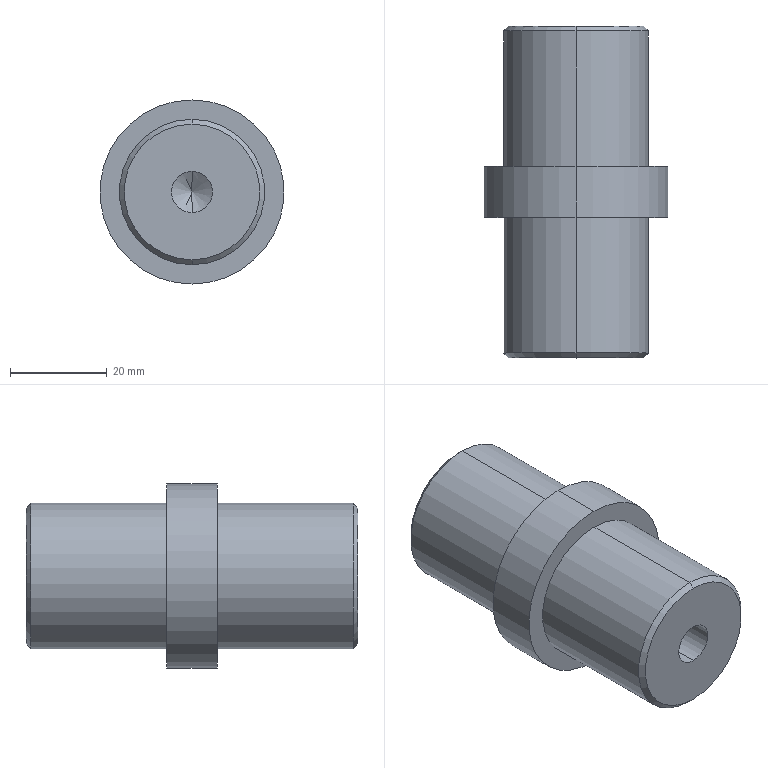Part | STEP file | PN_0010_default | 1 solid | 22 faces | box 38 x 68.5 x 38 mm | volume 49766 mm3 | cylinder 10 | cone 8 | plane 4 | commonest cylinder face diameters 8.5 x4 30 x4 38 x2
STEP:
#1=CARTESIAN_POINT('',(0.,0.,0.));
#2=DIRECTION('',(0.,0.,1.));
#3=DIRECTION('',(1.,0.,0.));
#4=AXIS2_PLACEMENT_3D('',#1,#2,#3);
#5=CARTESIAN_POINT('',(0.,-1.5,-4.25));
#6=VERTEX_POINT('',#5);
#7=CARTESIAN_POINT('',(0.,-29.,-4.25));
#8=VERTEX_POINT('',#7);
#9=CARTESIAN_POINT('',(0.,-29.,-4.25));
#10=DIRECTION('',(0.,-1.,0.));
#11=VECTOR('',#10,1.);
#12=LINE('',#9,#11);
#13=CARTESIAN_POINT('',(0.,-29.,0.));
#14=DIRECTION('',(0.,-1.,0.));
#15=DIRECTION('',(0.,0.,-1.));
#16=AXIS2_PLACEMENT_3D('',#13,#14,#15);
#17=CYLINDRICAL_SURFACE('',#16,4.25);
#18=CARTESIAN_POINT('',(6.283,0.));
#19=DIRECTION('',(0.,1.));
#20=VECTOR('',#19,1.);
#21=LINE('',#18,#20);
#22=(GEOMETRIC_REPRESENTATION_CONTEXT(2)PARAMETRIC_REPRESENTATION_CONTEXT()REPRESENTATION_CONTEXT('',''));
#23=DEFINITIONAL_REPRESENTATION('',(#21),#22);
#24=PCURVE('',#17,#23);
#25=CARTESIAN_POINT('',(0.,-29.,0.));
#26=DIRECTION('',(0.,-1.,0.));
#27=DIRECTION('',(0.,0.,-1.));
#28=AXIS2_PLACEMENT_3D('',#25,#26,#27);
#29=CYLINDRICAL_SURFACE('',#28,4.25);
#30=CARTESIAN_POINT('',(0.,0.));
#31=DIRECTION('',(0.,1.));
#32=VECTOR('',#31,1.);
#33=LINE('',#30,#32);
#34=(GEOMETRIC_REPRESENTATION_CONTEXT(2)PARAMETRIC_REPRESENTATION_CONTEXT()REPRESENTATION_CONTEXT('',''));
#35=DEFINITIONAL_REPRESENTATION('',(#33),#34);
#36=PCURVE('',#29,#35);
#37=SURFACE_CURVE('',#12,(#24,#36),.PCURVE_S1.);
#38=EDGE_CURVE('',#6,#8,#37,.T.);
#39=ORIENTED_EDGE('',*,*,#38,.T.);
#40=CARTESIAN_POINT('',(0.,-29.,4.25));
#41=VERTEX_POINT('',#40);
#42=CARTESIAN_POINT('',(0.,-29.,0.));
#43=DIRECTION('',(0.,-1.,0.));
#44=DIRECTION('',(0.,0.,-1.));
#45=AXIS2_PLACEMENT_3D('',#42,#43,#44);
#46=CIRCLE('',#45,4.25);
#47=CARTESIAN_POINT('',(0.,0.));
#48=DIRECTION('',(1.,0.));
#49=VECTOR('',#48,1.);
#50=LINE('',#47,#49);
#51=(GEOMETRIC_REPRESENTATION_CONTEXT(2)PARAMETRIC_REPRESENTATION_CONTEXT()REPRESENTATION_CONTEXT('',''));
#52=DEFINITIONAL_REPRESENTATION('',(#50),#51);
#53=PCURVE('',#17,#52);
#54=CARTESIAN_POINT('',(0.,-29.,0.));
#55=DIRECTION('',(0.,-1.,0.));
#56=DIRECTION('',(0.,0.,-1.));
#57=AXIS2_PLACEMENT_3D('',#54,#55,#56);
#58=PLANE('',#57);
#59=CARTESIAN_POINT('',(0.,0.));
#60=DIRECTION('',(1.,0.));
#61=AXIS2_PLACEMENT_2D('',#59,#60);
#62=CIRCLE('',#61,4.25);
#63=(GEOMETRIC_REPRESENTATION_CONTEXT(2)PARAMETRIC_REPRESENTATION_CONTEXT()REPRESENTATION_CONTEXT('',''));
#64=DEFINITIONAL_REPRESENTATION('',(#62),#63);
#65=PCURVE('',#58,#64);
#66=SURFACE_CURVE('',#46,(#53,#65),.PCURVE_S1.);
#67=EDGE_CURVE('',#41,#8,#66,.T.);
#68=ORIENTED_EDGE('',*,*,#67,.F.);
#69=CARTESIAN_POINT('',(0.,-1.5,4.25));
#70=VERTEX_POINT('',#69);
#71=CARTESIAN_POINT('',(0.,-29.,4.25));
#72=DIRECTION('',(0.,-1.,0.));
#73=VECTOR('',#72,1.);
#74=LINE('',#71,#73);
#75=CARTESIAN_POINT('',(3.142,0.));
#76=DIRECTION('',(0.,1.));
#77=VECTOR('',#76,1.);
#78=LINE('',#75,#77);
#79=(GEOMETRIC_REPRESENTATION_CONTEXT(2)PARAMETRIC_REPRESENTATION_CONTEXT()REPRESENTATION_CONTEXT('',''));
#80=DEFINITIONAL_REPRESENTATION('',(#78),#79);
#81=PCURVE('',#17,#80);
#82=CARTESIAN_POINT('',(3.142,0.));
#83=DIRECTION('',(0.,1.));
#84=VECTOR('',#83,1.);
#85=LINE('',#82,#84);
#86=(GEOMETRIC_REPRESENTATION_CONTEXT(2)PARAMETRIC_REPRESENTATION_CONTEXT()REPRESENTATION_CONTEXT('',''));
#87=DEFINITIONAL_REPRESENTATION('',(#85),#86);
#88=PCURVE('',#29,#87);
#89=SURFACE_CURVE('',#74,(#81,#88),.PCURVE_S1.);
#90=EDGE_CURVE('',#70,#41,#89,.T.);
#91=ORIENTED_EDGE('',*,*,#90,.F.);
#92=CARTESIAN_POINT('',(0.,-1.5,0.));
#93=DIRECTION('',(0.,-1.,0.));
#94=DIRECTION('',(0.,0.,-1.));
#95=AXIS2_PLACEMENT_3D('',#92,#93,#94);
#96=CIRCLE('',#95,4.25);
#97=CARTESIAN_POINT('',(0.,-27.5));
#98=DIRECTION('',(1.,0.));
#99=VECTOR('',#98,1.);
#100=LINE('',#97,#99);
#101=(GEOMETRIC_REPRESENTATION_CONTEXT(2)PARAMETRIC_REPRESENTATION_CONTEXT()REPRESENTATION_CONTEXT('',''));
#102=DEFINITIONAL_REPRESENTATION('',(#100),#101);
#103=PCURVE('',#17,#102);
#104=CARTESIAN_POINT('',(0.,-1.5,0.));
#105=DIRECTION('',(0.,-1.,0.));
#106=DIRECTION('',(0.,0.,-1.));
#107=AXIS2_PLACEMENT_3D('',#104,#105,#106);
#108=CONICAL_SURFACE('',#107,4.25,1.03);
#109=CARTESIAN_POINT('',(0.,0.));
#110=DIRECTION('',(1.,0.));
#111=VECTOR('',#110,1.);
#112=LINE('',#109,#111);
#113=(GEOMETRIC_REPRESENTATION_CONTEXT(2)PARAMETRIC_REPRESENTATION_CONTEXT()REPRESENTATION_CONTEXT('',''));
#114=DEFINITIONAL_REPRESENTATION('',(#112),#113);
#115=PCURVE('',#108,#114);
#116=SURFACE_CURVE('',#96,(#103,#115),.PCURVE_S1.);
#117=EDGE_CURVE('',#70,#6,#116,.T.);
#118=ORIENTED_EDGE('',*,*,#117,.T.);
#119=EDGE_LOOP('',(#39,#68,#91,#118));
#120=FACE_BOUND('',#119,.F.);
#121=ADVANCED_FACE('',(#120),#17,.F.);
#122=ORIENTED_EDGE('',*,*,#117,.F.);
#123=CARTESIAN_POINT('',(0.,1.054,0.));
#124=VERTEX_POINT('',#123);
#125=CARTESIAN_POINT('',(0.,-1.5,4.25));
#126=DIRECTION('',(0.,-0.515,0.8572));
#127=VECTOR('',#126,1.);
#128=LINE('',#125,#127);
#129=CARTESIAN_POINT('',(3.142,0.));
#130=DIRECTION('',(0.,1.));
#131=VECTOR('',#130,1.);
#132=LINE('',#129,#131);
#133=(GEOMETRIC_REPRESENTATION_CONTEXT(2)PARAMETRIC_REPRESENTATION_CONTEXT()REPRESENTATION_CONTEXT('',''));
#134=DEFINITIONAL_REPRESENTATION('',(#132),#133);
#135=PCURVE('',#108,#134);
#136=CARTESIAN_POINT('',(0.,-1.5,0.));
#137=DIRECTION('',(0.,-1.,0.));
#138=DIRECTION('',(0.,0.,-1.));
#139=AXIS2_PLACEMENT_3D('',#136,#137,#138);
#140=CONICAL_SURFACE('',#139,4.25,1.03);
#141=CARTESIAN_POINT('',(3.142,0.));
#142=DIRECTION('',(0.,1.));
#143=VECTOR('',#142,1.);
#144=LINE('',#141,#143);
#145=(GEOMETRIC_REPRESENTATION_CONTEXT(2)PARAMETRIC_REPRESENTATION_CONTEXT()REPRESENTATION_CONTEXT('',''));
#146=DEFINITIONAL_REPRESENTATION('',(#144),#145);
#147=PCURVE('',#140,#146);
#148=SURFACE_CURVE('',#128,(#135,#147),.PCURVE_S1.);
#149=EDGE_CURVE('',#124,#70,#148,.T.);
#150=ORIENTED_EDGE('',*,*,#149,.F.);
#151=CARTESIAN_POINT('',(0.,-1.5,-4.25));
#152=DIRECTION('',(0.,-0.515,-0.8572));
#153=VECTOR('',#152,1.);
#154=LINE('',#151,#153);
#155=CARTESIAN_POINT('',(6.283,0.));
#156=DIRECTION('',(0.,1.));
#157=VECTOR('',#156,1.);
#158=LINE('',#155,#157);
#159=(GEOMETRIC_REPRESENTATION_CONTEXT(2)PARAMETRIC_REPRESENTATION_CONTEXT()REPRESENTATION_CONTEXT('',''));
#160=DEFINITIONAL_REPRESENTATION('',(#158),#159);
#161=PCURVE('',#108,#160);
#162=CARTESIAN_POINT('',(0.,0.));
#163=DIRECTION('',(0.,1.));
#164=VECTOR('',#163,1.);
#165=LINE('',#162,#164);
#166=(GEOMETRIC_REPRESENTATION_CONTEXT(2)PARAMETRIC_REPRESENTATION_CONTEXT()REPRESENTATION_CONTEXT('',''));
#167=DEFINITIONAL_REPRESENTATION('',(#165),#166);
#168=PCURVE('',#140,#167);
#169=SURFACE_CURVE('',#154,(#161,#168),.PCURVE_S1.);
#170=EDGE_CURVE('',#124,#6,#169,.T.);
#171=ORIENTED_EDGE('',*,*,#170,.T.);
#172=EDGE_LOOP('',(#122,#150,#171));
#173=FACE_BOUND('',#172,.F.);
#174=ADVANCED_FACE('',(#173),#108,.F.);
#175=CARTESIAN_POINT('',(0.,15.,4.25));
#176=VERTEX_POINT('',#175);
#177=CARTESIAN_POINT('',(0.,39.5,4.25));
#178=VERTEX_POINT('',#177);
#179=CARTESIAN_POINT('',(0.,39.5,4.25));
#180=DIRECTION('',(0.,1.,0.));
#181=VECTOR('',#180,1.);
#182=LINE('',#179,#181);
#183=CARTESIAN_POINT('',(0.,39.5,0.));
#184=DIRECTION('',(0.,1.,0.));
#185=DIRECTION('',(0.,0.,1.));
#186=AXIS2_PLACEMENT_3D('',#183,#184,#185);
#187=CYLINDRICAL_SURFACE('',#186,4.25);
#188=CARTESIAN_POINT('',(6.283,0.));
#189=DIRECTION('',(0.,1.));
#190=VECTOR('',#189,1.);
#191=LINE('',#188,#190);
#192=(GEOMETRIC_REPRESENTATION_CONTEXT(2)PARAMETRIC_REPRESENTATION_CONTEXT()REPRESENTATION_CONTEXT('',''));
#193=DEFINITIONAL_REPRESENTATION('',(#191),#192);
#194=PCURVE('',#187,#193);
#195=CARTESIAN_POINT('',(0.,39.5,0.));
#196=DIRECTION('',(0.,1.,0.));
#197=DIRECTION('',(0.,0.,1.));
#198=AXIS2_PLACEMENT_3D('',#195,#196,#197);
#199=CYLINDRICAL_SURFACE('',#198,4.25);
#200=CARTESIAN_POINT('',(0.,0.));
#201=DIRECTION('',(0.,1.));
#202=VECTOR('',#201,1.);
#203=LINE('',#200,#202);
#204=(GEOMETRIC_REPRESENTATION_CONTEXT(2)PARAMETRIC_REPRESENTATION_CONTEXT()REPRESENTATION_CONTEXT('',''));
#205=DEFINITIONAL_REPRESENTATION('',(#203),#204);
#206=PCURVE('',#199,#205);
#207=SURFACE_CURVE('',#182,(#194,#206),.PCURVE_S1.);
#208=EDGE_CURVE('',#176,#178,#207,.T.);
#209=ORIENTED_EDGE('',*,*,#208,.T.);
#210=CARTESIAN_POINT('',(0.,39.5,-4.25));
#211=VERTEX_POINT('',#210);
#212=CARTESIAN_POINT('',(0.,39.5,0.));
#213=DIRECTION('',(0.,1.,0.));
#214=DIRECTION('',(0.,0.,1.));
#215=AXIS2_PLACEMENT_3D('',#212,#213,#214);
#216=CIRCLE('',#215,4.25);
#217=CARTESIAN_POINT('',(0.,0.));
#218=DIRECTION('',(1.,0.));
#219=VECTOR('',#218,1.);
#220=LINE('',#217,#219);
#221=(GEOMETRIC_REPRESENTATION_CONTEXT(2)PARAMETRIC_REPRESENTATION_CONTEXT()REPRESENTATION_CONTEXT('',''));
#222=DEFINITIONAL_REPRESENTATION('',(#220),#221);
#223=PCURVE('',#187,#222);
#224=CARTESIAN_POINT('',(0.,39.5,0.));
#225=DIRECTION('',(0.,1.,0.));
#226=DIRECTION('',(0.,0.,1.));
#227=AXIS2_PLACEMENT_3D('',#224,#225,#226);
#228=PLANE('',#227);
#229=CARTESIAN_POINT('',(0.,0.));
#230=DIRECTION('',(1.,0.));
#231=AXIS2_PLACEMENT_2D('',#229,#230);
#232=CIRCLE('',#231,4.25);
#233=(GEOMETRIC_REPRESENTATION_CONTEXT(2)PARAMETRIC_REPRESENTATION_CONTEXT()REPRESENTATION_CONTEXT('',''));
#234=DEFINITIONAL_REPRESENTATION('',(#232),#233);
#235=PCURVE('',#228,#234);
#236=SURFACE_CURVE('',#216,(#223,#235),.PCURVE_S1.);
#237=EDGE_CURVE('',#211,#178,#236,.T.);
#238=ORIENTED_EDGE('',*,*,#237,.F.);
#239=CARTESIAN_POINT('',(0.,15.,-4.25));
#240=VERTEX_POINT('',#239);
#241=CARTESIAN_POINT('',(0.,39.5,-4.25));
#242=DIRECTION('',(0.,1.,0.));
#243=VECTOR('',#242,1.);
#244=LINE('',#241,#243);
#245=CARTESIAN_POINT('',(3.142,0.));
#246=DIRECTION('',(0.,1.));
#247=VECTOR('',#246,1.);
#248=LINE('',#245,#247);
#249=(GEOMETRIC_REPRESENTATION_CONTEXT(2)PARAMETRIC_REPRESENTATION_CONTEXT()REPRESENTATION_CONTEXT('',''));
#250=DEFINITIONAL_REPRESENTATION('',(#248),#249);
#251=PCURVE('',#187,#250);
#252=CARTESIAN_POINT('',(3.142,0.));
#253=DIRECTION('',(0.,1.));
#254=VECTOR('',#253,1.);
#255=LINE('',#252,#254);
#256=(GEOMETRIC_REPRESENTATION_CONTEXT(2)PARAMETRIC_REPRESENTATION_CONTEXT()REPRESENTATION_CONTEXT('',''));
#257=DEFINITIONAL_REPRESENTATION('',(#255),#256);
#258=PCURVE('',#199,#257);
#259=SURFACE_CURVE('',#244,(#251,#258),.PCURVE_S1.);
#260=EDGE_CURVE('',#240,#211,#259,.T.);
#261=ORIENTED_EDGE('',*,*,#260,.F.);
#262=CARTESIAN_POINT('',(0.,15.,0.));
#263=DIRECTION('',(0.,1.,0.));
#264=DIRECTION('',(0.,0.,1.));
#265=AXIS2_PLACEMENT_3D('',#262,#263,#264);
#266=CIRCLE('',#265,4.25);
#267=CARTESIAN_POINT('',(0.,-24.5));
#268=DIRECTION('',(1.,0.));
#269=VECTOR('',#268,1.);
#270=LINE('',#267,#269);
#271=(GEOMETRIC_REPRESENTATION_CONTEXT(2)PARAMETRIC_REPRESENTATION_CONTEXT()REPRESENTATION_CONTEXT('',''));
#272=DEFINITIONAL_REPRESENTATION('',(#270),#271);
#273=PCURVE('',#187,#272);
#274=CARTESIAN_POINT('',(0.,15.,0.));
#275=DIRECTION('',(0.,1.,0.));
#276=DIRECTION('',(0.,0.,1.));
#277=AXIS2_PLACEMENT_3D('',#274,#275,#276);
#278=CONICAL_SURFACE('',#277,4.25,1.03);
#279=CARTESIAN_POINT('',(0.,0.));
#280=DIRECTION('',(1.,0.));
#281=VECTOR('',#280,1.);
#282=LINE('',#279,#281);
#283=(GEOMETRIC_REPRESENTATION_CONTEXT(2)PARAMETRIC_REPRESENTATION_CONTEXT()REPRESENTATION_CONTEXT('',''));
#284=DEFINITIONAL_REPRESENTATION('',(#282),#283);
#285=PCURVE('',#278,#284);
#286=SURFACE_CURVE('',#266,(#273,#285),.PCURVE_S1.);
#287=EDGE_CURVE('',#240,#176,#286,.T.);
#288=ORIENTED_EDGE('',*,*,#287,.T.);
#289=EDGE_LOOP('',(#209,#238,#261,#288));
#290=FACE_BOUND('',#289,.F.);
#291=ADVANCED_FACE('',(#290),#187,.F.);
#292=ORIENTED_EDGE('',*,*,#287,.F.);
#293=CARTESIAN_POINT('',(0.,12.446,0.));
#294=VERTEX_POINT('',#293);
#295=CARTESIAN_POINT('',(0.,15.,-4.25));
#296=DIRECTION('',(0.,0.515,-0.8572));
#297=VECTOR('',#296,1.);
#298=LINE('',#295,#297);
#299=CARTESIAN_POINT('',(3.142,0.));
#300=DIRECTION('',(0.,1.));
#301=VECTOR('',#300,1.);
#302=LINE('',#299,#301);
#303=(GEOMETRIC_REPRESENTATION_CONTEXT(2)PARAMETRIC_REPRESENTATION_CONTEXT()REPRESENTATION_CONTEXT('',''));
#304=DEFINITIONAL_REPRESENTATION('',(#302),#303);
#305=PCURVE('',#278,#304);
#306=CARTESIAN_POINT('',(0.,15.,0.));
#307=DIRECTION('',(0.,1.,0.));
#308=DIRECTION('',(0.,0.,1.));
#309=AXIS2_PLACEMENT_3D('',#306,#307,#308);
#310=CONICAL_SURFACE('',#309,4.25,1.03);
#311=CARTESIAN_POINT('',(3.142,0.));
#312=DIRECTION('',(0.,1.));
#313=VECTOR('',#312,1.);
#314=LINE('',#311,#313);
#315=(GEOMETRIC_REPRESENTATION_CONTEXT(2)PARAMETRIC_REPRESENTATION_CONTEXT()REPRESENTATION_CONTEXT('',''));
#316=DEFINITIONAL_REPRESENTATION('',(#314),#315);
#317=PCURVE('',#310,#316);
#318=SURFACE_CURVE('',#298,(#305,#317),.PCURVE_S1.);
#319=EDGE_CURVE('',#294,#240,#318,.T.);
#320=ORIENTED_EDGE('',*,*,#319,.F.);
#321=CARTESIAN_POINT('',(0.,15.,4.25));
#322=DIRECTION('',(0.,0.515,0.8572));
#323=VECTOR('',#322,1.);
#324=LINE('',#321,#323);
#325=CARTESIAN_POINT('',(6.283,0.));
#326=DIRECTION('',(0.,1.));
#327=VECTOR('',#326,1.);
#328=LINE('',#325,#327);
#329=(GEOMETRIC_REPRESENTATION_CONTEXT(2)PARAMETRIC_REPRESENTATION_CONTEXT()REPRESENTATION_CONTEXT('',''));
#330=DEFINITIONAL_REPRESENTATION('',(#328),#329);
#331=PCURVE('',#278,#330);
#332=CARTESIAN_POINT('',(0.,0.));
#333=DIRECTION('',(0.,1.));
#334=VECTOR('',#333,1.);
#335=LINE('',#332,#334);
#336=(GEOMETRIC_REPRESENTATION_CONTEXT(2)PARAMETRIC_REPRESENTATION_CONTEXT()REPRESENTATION_CONTEXT('',''));
#337=DEFINITIONAL_REPRESENTATION('',(#335),#336);
#338=PCURVE('',#310,#337);
#339=SURFACE_CURVE('',#324,(#331,#338),.PCURVE_S1.);
#340=EDGE_CURVE('',#294,#176,#339,.T.);
#341=ORIENTED_EDGE('',*,*,#340,.T.);
#342=EDGE_LOOP('',(#292,#320,#341));
#343=FACE_BOUND('',#342,.F.);
#344=ADVANCED_FACE('',(#343),#278,.F.);
#345=CARTESIAN_POINT('',(0.,-29.,-14.));
#346=VERTEX_POINT('',#345);
#347=CARTESIAN_POINT('',(0.,-29.,14.));
#348=VERTEX_POINT('',#347);
#349=CARTESIAN_POINT('',(0.,-29.,0.));
#350=DIRECTION('',(0.,-1.,0.));
#351=DIRECTION('',(0.,0.,-1.));
#352=AXIS2_PLACEMENT_3D('',#349,#350,#351);
#353=CIRCLE('',#352,14.);
#354=CARTESIAN_POINT('',(0.,-29.,0.));
#355=DIRECTION('',(0.,1.,0.));
#356=DIRECTION('',(0.,0.,1.));
#357=AXIS2_PLACEMENT_3D('',#354,#355,#356);
#358=CONICAL_SURFACE('',#357,14.,0.7854);
#359=CARTESIAN_POINT('',(3.142,0.));
#360=DIRECTION('',(-1.,0.));
#361=VECTOR('',#360,1.);
#362=LINE('',#359,#361);
#363=(GEOMETRIC_REPRESENTATION_CONTEXT(2)PARAMETRIC_REPRESENTATION_CONTEXT()REPRESENTATION_CONTEXT('',''));
#364=DEFINITIONAL_REPRESENTATION('',(#362),#363);
#365=PCURVE('',#358,#364);
#366=CARTESIAN_POINT('',(0.,0.));
#367=DIRECTION('',(1.,0.));
#368=AXIS2_PLACEMENT_2D('',#366,#367);
#369=CIRCLE('',#368,14.);
#370=(GEOMETRIC_REPRESENTATION_CONTEXT(2)PARAMETRIC_REPRESENTATION_CONTEXT()REPRESENTATION_CONTEXT('',''));
#371=DEFINITIONAL_REPRESENTATION('',(#369),#370);
#372=PCURVE('',#58,#371);
#373=SURFACE_CURVE('',#353,(#365,#372),.PCURVE_S1.);
#374=EDGE_CURVE('',#346,#348,#373,.T.);
#375=ORIENTED_EDGE('',*,*,#374,.F.);
#376=CARTESIAN_POINT('',(0.,-28.,-15.));
#377=VERTEX_POINT('',#376);
#378=CARTESIAN_POINT('',(0.,-29.,-14.));
#379=DIRECTION('',(0.,0.7071,-0.7071));
#380=VECTOR('',#379,1.);
#381=LINE('',#378,#380);
#382=CARTESIAN_POINT('',(3.142,0.));
#383=DIRECTION('',(0.,1.));
#384=VECTOR('',#383,1.);
#385=LINE('',#382,#384);
#386=(GEOMETRIC_REPRESENTATION_CONTEXT(2)PARAMETRIC_REPRESENTATION_CONTEXT()REPRESENTATION_CONTEXT('',''));
#387=DEFINITIONAL_REPRESENTATION('',(#385),#386);
#388=PCURVE('',#358,#387);
#389=CARTESIAN_POINT('',(0.,-29.,0.));
#390=DIRECTION('',(0.,1.,0.));
#391=DIRECTION('',(0.,0.,1.));
#392=AXIS2_PLACEMENT_3D('',#389,#390,#391);
#393=CONICAL_SURFACE('',#392,14.,0.7854);
#394=CARTESIAN_POINT('',(3.142,0.));
#395=DIRECTION('',(0.,1.));
#396=VECTOR('',#395,1.);
#397=LINE('',#394,#396);
#398=(GEOMETRIC_REPRESENTATION_CONTEXT(2)PARAMETRIC_REPRESENTATION_CONTEXT()REPRESENTATION_CONTEXT('',''));
#399=DEFINITIONAL_REPRESENTATION('',(#397),#398);
#400=PCURVE('',#393,#399);
#401=SURFACE_CURVE('',#381,(#388,#400),.PCURVE_S1.);
#402=EDGE_CURVE('',#346,#377,#401,.T.);
#403=ORIENTED_EDGE('',*,*,#402,.T.);
#404=CARTESIAN_POINT('',(0.,-28.,15.));
#405=VERTEX_POINT('',#404);
#406=CARTESIAN_POINT('',(0.,-28.,0.));
#407=DIRECTION('',(0.,1.,0.));
#408=DIRECTION('',(0.,0.,-1.));
#409=AXIS2_PLACEMENT_3D('',#406,#407,#408);
#410=CIRCLE('',#409,15.);
#411=CARTESIAN_POINT('',(-3.142,1.));
#412=DIRECTION('',(1.,0.));
#413=VECTOR('',#412,1.);
#414=LINE('',#411,#413);
#415=(GEOMETRIC_REPRESENTATION_CONTEXT(2)PARAMETRIC_REPRESENTATION_CONTEXT()REPRESENTATION_CONTEXT('',''));
#416=DEFINITIONAL_REPRESENTATION('',(#414),#415);
#417=PCURVE('',#358,#416);
#418=CARTESIAN_POINT('',(0.,-29.,0.));
#419=DIRECTION('',(0.,1.,0.));
#420=DIRECTION('',(0.,0.,1.));
#421=AXIS2_PLACEMENT_3D('',#418,#419,#420);
#422=CYLINDRICAL_SURFACE('',#421,15.);
#423=CARTESIAN_POINT('',(-3.142,1.));
#424=DIRECTION('',(1.,0.));
#425=VECTOR('',#424,1.);
#426=LINE('',#423,#425);
#427=(GEOMETRIC_REPRESENTATION_CONTEXT(2)PARAMETRIC_REPRESENTATION_CONTEXT()REPRESENTATION_CONTEXT('',''));
#428=DEFINITIONAL_REPRESENTATION('',(#426),#427);
#429=PCURVE('',#422,#428);
#430=SURFACE_CURVE('',#410,(#417,#429),.PCURVE_S1.);
#431=EDGE_CURVE('',#405,#377,#430,.T.);
#432=ORIENTED_EDGE('',*,*,#431,.F.);
#433=CARTESIAN_POINT('',(0.,-29.,14.));
#434=DIRECTION('',(0.,0.7071,0.7071));
#435=VECTOR('',#434,1.);
#436=LINE('',#433,#435);
#437=CARTESIAN_POINT('',(0.,0.));
#438=DIRECTION('',(0.,1.));
#439=VECTOR('',#438,1.);
#440=LINE('',#437,#439);
#441=(GEOMETRIC_REPRESENTATION_CONTEXT(2)PARAMETRIC_REPRESENTATION_CONTEXT()REPRESENTATION_CONTEXT('',''));
#442=DEFINITIONAL_REPRESENTATION('',(#440),#441);
#443=PCURVE('',#358,#442);
#444=CARTESIAN_POINT('',(6.283,0.));
#445=DIRECTION('',(0.,1.));
#446=VECTOR('',#445,1.);
#447=LINE('',#444,#446);
#448=(GEOMETRIC_REPRESENTATION_CONTEXT(2)PARAMETRIC_REPRESENTATION_CONTEXT()REPRESENTATION_CONTEXT('',''));
#449=DEFINITIONAL_REPRESENTATION('',(#447),#448);
#450=PCURVE('',#393,#449);
#451=SURFACE_CURVE('',#436,(#443,#450),.PCURVE_S1.);
#452=EDGE_CURVE('',#348,#405,#451,.T.);
#453=ORIENTED_EDGE('',*,*,#452,.F.);
#454=EDGE_LOOP('',(#375,#403,#432,#453));
#455=FACE_BOUND('',#454,.T.);
#456=ADVANCED_FACE('',(#455),#358,.T.);
#457=CARTESIAN_POINT('',(0.,39.5,14.));
#458=VERTEX_POINT('',#457);
#459=CARTESIAN_POINT('',(0.,39.5,-14.));
#460=VERTEX_POINT('',#459);
#461=CARTESIAN_POINT('',(0.,39.5,0.));
#462=DIRECTION('',(0.,1.,0.));
#463=DIRECTION('',(0.,0.,1.));
#464=AXIS2_PLACEMENT_3D('',#461,#462,#463);
#465=CIRCLE('',#464,14.);
#466=CARTESIAN_POINT('',(0.,39.5,0.));
#467=DIRECTION('',(0.,-1.,0.));
#468=DIRECTION('',(0.,0.,-1.));
#469=AXIS2_PLACEMENT_3D('',#466,#467,#468);
#470=CONICAL_SURFACE('',#469,14.,0.7854);
#471=CARTESIAN_POINT('',(3.142,0.));
#472=DIRECTION('',(-1.,0.));
#473=VECTOR('',#472,1.);
#474=LINE('',#471,#473);
#475=(GEOMETRIC_REPRESENTATION_CONTEXT(2)PARAMETRIC_REPRESENTATION_CONTEXT()REPRESENTATION_CONTEXT('',''));
#476=DEFINITIONAL_REPRESENTATION('',(#474),#475);
#477=PCURVE('',#470,#476);
#478=CARTESIAN_POINT('',(0.,0.));
#479=DIRECTION('',(1.,0.));
#480=AXIS2_PLACEMENT_2D('',#478,#479);
#481=CIRCLE('',#480,14.);
#482=(GEOMETRIC_REPRESENTATION_CONTEXT(2)PARAMETRIC_REPRESENTATION_CONTEXT()REPRESENTATION_CONTEXT('',''));
#483=DEFINITIONAL_REPRESENTATION('',(#481),#482);
#484=PCURVE('',#228,#483);
#485=SURFACE_CURVE('',#465,(#477,#484),.PCURVE_S1.);
#486=EDGE_CURVE('',#458,#460,#485,.T.);
#487=ORIENTED_EDGE('',*,*,#486,.F.);
#488=CARTESIAN_POINT('',(0.,38.5,15.));
#489=VERTEX_POINT('',#488);
#490=CARTESIAN_POINT('',(0.,39.5,14.));
#491=DIRECTION('',(0.,-0.7071,0.7071));
#492=VECTOR('',#491,1.);
#493=LINE('',#490,#492);
#494=CARTESIAN_POINT('',(3.142,0.));
#495=DIRECTION('',(0.,1.));
#496=VECTOR('',#495,1.);
#497=LINE('',#494,#496);
#498=(GEOMETRIC_REPRESENTATION_CONTEXT(2)PARAMETRIC_REPRESENTATION_CONTEXT()REPRESENTATION_CONTEXT('',''));
#499=DEFINITIONAL_REPRESENTATION('',(#497),#498);
#500=PCURVE('',#470,#499);
#501=CARTESIAN_POINT('',(0.,39.5,0.));
#502=DIRECTION('',(0.,-1.,0.));
#503=DIRECTION('',(0.,0.,-1.));
#504=AXIS2_PLACEMENT_3D('',#501,#502,#503);
#505=CONICAL_SURFACE('',#504,14.,0.7854);
#506=CARTESIAN_POINT('',(3.142,0.));
#507=DIRECTION('',(0.,1.));
#508=VECTOR('',#507,1.);
#509=LINE('',#506,#508);
#510=(GEOMETRIC_REPRESENTATION_CONTEXT(2)PARAMETRIC_REPRESENTATION_CONTEXT()REPRESENTATION_CONTEXT('',''));
#511=DEFINITIONAL_REPRESENTATION('',(#509),#510);
#512=PCURVE('',#505,#511);
#513=SURFACE_CURVE('',#493,(#500,#512),.PCURVE_S1.);
#514=EDGE_CURVE('',#458,#489,#513,.T.);
#515=ORIENTED_EDGE('',*,*,#514,.T.);
#516=CARTESIAN_POINT('',(0.,38.5,-15.));
#517=VERTEX_POINT('',#516);
#518=CARTESIAN_POINT('',(0.,38.5,0.));
#519=DIRECTION('',(0.,-1.,0.));
#520=DIRECTION('',(0.,0.,1.));
#521=AXIS2_PLACEMENT_3D('',#518,#519,#520);
#522=CIRCLE('',#521,15.);
#523=CARTESIAN_POINT('',(-3.142,1.));
#524=DIRECTION('',(1.,0.));
#525=VECTOR('',#524,1.);
#526=LINE('',#523,#525);
#527=(GEOMETRIC_REPRESENTATION_CONTEXT(2)PARAMETRIC_REPRESENTATION_CONTEXT()REPRESENTATION_CONTEXT('',''));
#528=DEFINITIONAL_REPRESENTATION('',(#526),#527);
#529=PCURVE('',#470,#528);
#530=CARTESIAN_POINT('',(0.,39.5,0.));
#531=DIRECTION('',(0.,-1.,0.));
#532=DIRECTION('',(0.,0.,-1.));
#533=AXIS2_PLACEMENT_3D('',#530,#531,#532);
#534=CYLINDRICAL_SURFACE('',#533,15.);
#535=CARTESIAN_POINT('',(-3.142,1.));
#536=DIRECTION('',(1.,0.));
#537=VECTOR('',#536,1.);
#538=LINE('',#535,#537);
#539=(GEOMETRIC_REPRESENTATION_CONTEXT(2)PARAMETRIC_REPRESENTATION_CONTEXT()REPRESENTATION_CONTEXT('',''));
#540=DEFINITIONAL_REPRESENTATION('',(#538),#539);
#541=PCURVE('',#534,#540);
#542=SURFACE_CURVE('',#522,(#529,#541),.PCURVE_S1.);
#543=EDGE_CURVE('',#517,#489,#542,.T.);
#544=ORIENTED_EDGE('',*,*,#543,.F.);
#545=CARTESIAN_POINT('',(0.,39.5,-14.));
#546=DIRECTION('',(0.,-0.7071,-0.7071));
#547=VECTOR('',#546,1.);
#548=LINE('',#545,#547);
#549=CARTESIAN_POINT('',(0.,0.));
#550=DIRECTION('',(0.,1.));
#551=VECTOR('',#550,1.);
#552=LINE('',#549,#551);
#553=(GEOMETRIC_REPRESENTATION_CONTEXT(2)PARAMETRIC_REPRESENTATION_CONTEXT()REPRESENTATION_CONTEXT('',''));
#554=DEFINITIONAL_REPRESENTATION('',(#552),#553);
#555=PCURVE('',#470,#554);
#556=CARTESIAN_POINT('',(6.283,0.));
#557=DIRECTION('',(0.,1.));
#558=VECTOR('',#557,1.);
#559=LINE('',#556,#558);
#560=(GEOMETRIC_REPRESENTATION_CONTEXT(2)PARAMETRIC_REPRESENTATION_CONTEXT()REPRESENTATION_CONTEXT('',''));
#561=DEFINITIONAL_REPRESENTATION('',(#559),#560);
#562=PCURVE('',#505,#561);
#563=SURFACE_CURVE('',#548,(#555,#562),.PCURVE_S1.);
#564=EDGE_CURVE('',#460,#517,#563,.T.);
#565=ORIENTED_EDGE('',*,*,#564,.F.);
#566=EDGE_LOOP('',(#487,#515,#544,#565));
#567=FACE_BOUND('',#566,.T.);
#568=ADVANCED_FACE('',(#567),#470,.T.);
#569=ORIENTED_EDGE('',*,*,#431,.T.);
#570=CARTESIAN_POINT('',(0.,0.,-15.));
#571=VERTEX_POINT('',#570);
#572=CARTESIAN_POINT('',(0.,-29.,-15.));
#573=DIRECTION('',(0.,1.,0.));
#574=VECTOR('',#573,1.);
#575=LINE('',#572,#574);
#576=CARTESIAN_POINT('',(3.142,0.));
#577=DIRECTION('',(0.,1.));
#578=VECTOR('',#577,1.);
#579=LINE('',#576,#578);
#580=(GEOMETRIC_REPRESENTATION_CONTEXT(2)PARAMETRIC_REPRESENTATION_CONTEXT()REPRESENTATION_CONTEXT('',''));
#581=DEFINITIONAL_REPRESENTATION('',(#579),#580);
#582=PCURVE('',#422,#581);
#583=CARTESIAN_POINT('',(0.,-29.,0.));
#584=DIRECTION('',(0.,1.,0.));
#585=DIRECTION('',(0.,0.,1.));
#586=AXIS2_PLACEMENT_3D('',#583,#584,#585);
#587=CYLINDRICAL_SURFACE('',#586,15.);
#588=CARTESIAN_POINT('',(3.142,0.));
#589=DIRECTION('',(0.,1.));
#590=VECTOR('',#589,1.);
#591=LINE('',#588,#590);
#592=(GEOMETRIC_REPRESENTATION_CONTEXT(2)PARAMETRIC_REPRESENTATION_CONTEXT()REPRESENTATION_CONTEXT('',''));
#593=DEFINITIONAL_REPRESENTATION('',(#591),#592);
#594=PCURVE('',#587,#593);
#595=SURFACE_CURVE('',#575,(#582,#594),.PCURVE_S1.);
#596=EDGE_CURVE('',#377,#571,#595,.T.);
#597=ORIENTED_EDGE('',*,*,#596,.T.);
#598=CARTESIAN_POINT('',(0.,0.,15.));
#599=VERTEX_POINT('',#598);
#600=CARTESIAN_POINT('',(0.,0.,0.));
#601=DIRECTION('',(0.,-1.,0.));
#602=DIRECTION('',(0.,0.,1.));
#603=AXIS2_PLACEMENT_3D('',#600,#601,#602);
#604=CIRCLE('',#603,15.);
#605=CARTESIAN_POINT('',(6.283,29.));
#606=DIRECTION('',(-1.,0.));
#607=VECTOR('',#606,1.);
#608=LINE('',#605,#607);
#609=(GEOMETRIC_REPRESENTATION_CONTEXT(2)PARAMETRIC_REPRESENTATION_CONTEXT()REPRESENTATION_CONTEXT('',''));
#610=DEFINITIONAL_REPRESENTATION('',(#608),#609);
#611=PCURVE('',#422,#610);
#612=CARTESIAN_POINT('',(0.,0.,0.));
#613=DIRECTION('',(0.,1.,0.));
#614=DIRECTION('',(0.,0.,1.));
#615=AXIS2_PLACEMENT_3D('',#612,#613,#614);
#616=PLANE('',#615);
#617=CARTESIAN_POINT('',(15.,0.));
#618=CARTESIAN_POINT('',(15.,-25.981));
#619=CARTESIAN_POINT('',(-7.5,-12.99));
#620=CARTESIAN_POINT('',(-30.,0.));
#621=CARTESIAN_POINT('',(-7.5,12.99));
#622=CARTESIAN_POINT('',(15.,25.981));
#623=CARTESIAN_POINT('',(15.,0.));
#624=(BOUNDED_CURVE()B_SPLINE_CURVE(2,(#617,#618,#619,#620,#621,#622,#623),.UNSPECIFIED.,.T.,.F.)B_SPLINE_CURVE_WITH_KNOTS((1,2,2,2,2,1),(-2.094,0.,2.094,4.189,6.283,8.378),.UNSPECIFIED.)CURVE()GEOMETRIC_REPRESENTATION_ITEM()RATIONAL_B_SPLINE_CURVE((1.,0.5,1.,0.5,1.,0.5,1.))REPRESENTATION_ITEM(''));
#625=(GEOMETRIC_REPRESENTATION_CONTEXT(2)PARAMETRIC_REPRESENTATION_CONTEXT()REPRESENTATION_CONTEXT('',''));
#626=DEFINITIONAL_REPRESENTATION('',(#624),#625);
#627=PCURVE('',#616,#626);
#628=SURFACE_CURVE('',#604,(#611,#627),.PCURVE_S1.);
#629=EDGE_CURVE('',#571,#599,#628,.T.);
#630=ORIENTED_EDGE('',*,*,#629,.T.);
#631=CARTESIAN_POINT('',(0.,-29.,15.));
#632=DIRECTION('',(0.,1.,0.));
#633=VECTOR('',#632,1.);
#634=LINE('',#631,#633);
#635=CARTESIAN_POINT('',(0.,0.));
#636=DIRECTION('',(0.,1.));
#637=VECTOR('',#636,1.);
#638=LINE('',#635,#637);
#639=(GEOMETRIC_REPRESENTATION_CONTEXT(2)PARAMETRIC_REPRESENTATION_CONTEXT()REPRESENTATION_CONTEXT('',''));
#640=DEFINITIONAL_REPRESENTATION('',(#638),#639);
#641=PCURVE('',#422,#640);
#642=CARTESIAN_POINT('',(6.283,0.));
#643=DIRECTION('',(0.,1.));
#644=VECTOR('',#643,1.);
#645=LINE('',#642,#644);
#646=(GEOMETRIC_REPRESENTATION_CONTEXT(2)PARAMETRIC_REPRESENTATION_CONTEXT()REPRESENTATION_CONTEXT('',''));
#647=DEFINITIONAL_REPRESENTATION('',(#645),#646);
#648=PCURVE('',#587,#647);
#649=SURFACE_CURVE('',#634,(#641,#648),.PCURVE_S1.);
#650=EDGE_CURVE('',#405,#599,#649,.T.);
#651=ORIENTED_EDGE('',*,*,#650,.F.);
#652=EDGE_LOOP('',(#569,#597,#630,#651));
#653=FACE_BOUND('',#652,.T.);
#654=ADVANCED_FACE('',(#653),#422,.T.);
#655=ORIENTED_EDGE('',*,*,#543,.T.);
#656=CARTESIAN_POINT('',(0.,10.5,15.));
#657=VERTEX_POINT('',#656);
#658=CARTESIAN_POINT('',(0.,39.5,15.));
#659=DIRECTION('',(0.,-1.,0.));
#660=VECTOR('',#659,1.);
#661=LINE('',#658,#660);
#662=CARTESIAN_POINT('',(3.142,0.));
#663=DIRECTION('',(0.,1.));
#664=VECTOR('',#663,1.);
#665=LINE('',#662,#664);
#666=(GEOMETRIC_REPRESENTATION_CONTEXT(2)PARAMETRIC_REPRESENTATION_CONTEXT()REPRESENTATION_CONTEXT('',''));
#667=DEFINITIONAL_REPRESENTATION('',(#665),#666);
#668=PCURVE('',#534,#667);
#669=CARTESIAN_POINT('',(0.,39.5,0.));
#670=DIRECTION('',(0.,-1.,0.));
#671=DIRECTION('',(0.,0.,-1.));
#672=AXIS2_PLACEMENT_3D('',#669,#670,#671);
#673=CYLINDRICAL_SURFACE('',#672,15.);
#674=CARTESIAN_POINT('',(3.142,0.));
#675=DIRECTION('',(0.,1.));
#676=VECTOR('',#675,1.);
#677=LINE('',#674,#676);
#678=(GEOMETRIC_REPRESENTATION_CONTEXT(2)PARAMETRIC_REPRESENTATION_CONTEXT()REPRESENTATION_CONTEXT('',''));
#679=DEFINITIONAL_REPRESENTATION('',(#677),#678);
#680=PCURVE('',#673,#679);
#681=SURFACE_CURVE('',#661,(#668,#680),.PCURVE_S1.);
#682=EDGE_CURVE('',#489,#657,#681,.T.);
#683=ORIENTED_EDGE('',*,*,#682,.T.);
#684=CARTESIAN_POINT('',(0.,10.5,-15.));
#685=VERTEX_POINT('',#684);
#686=CARTESIAN_POINT('',(0.,10.5,0.));
#687=DIRECTION('',(0.,1.,0.));
#688=DIRECTION('',(0.,0.,1.));
#689=AXIS2_PLACEMENT_3D('',#686,#687,#688);
#690=CIRCLE('',#689,15.);
#691=CARTESIAN_POINT('',(3.142,29.));
#692=DIRECTION('',(-1.,0.));
#693=VECTOR('',#692,1.);
#694=LINE('',#691,#693);
#695=(GEOMETRIC_REPRESENTATION_CONTEXT(2)PARAMETRIC_REPRESENTATION_CONTEXT()REPRESENTATION_CONTEXT('',''));
#696=DEFINITIONAL_REPRESENTATION('',(#694),#695);
#697=PCURVE('',#534,#696);
#698=CARTESIAN_POINT('',(0.,10.5,0.));
#699=DIRECTION('',(0.,1.,0.));
#700=DIRECTION('',(0.,0.,1.));
#701=AXIS2_PLACEMENT_3D('',#698,#699,#700);
#702=PLANE('',#701);
#703=CARTESIAN_POINT('',(0.,0.));
#704=DIRECTION('',(1.,0.));
#705=AXIS2_PLACEMENT_2D('',#703,#704);
#706=CIRCLE('',#705,15.);
#707=(GEOMETRIC_REPRESENTATION_CONTEXT(2)PARAMETRIC_REPRESENTATION_CONTEXT()REPRESENTATION_CONTEXT('',''));
#708=DEFINITIONAL_REPRESENTATION('',(#706),#707);
#709=PCURVE('',#702,#708);
#710=SURFACE_CURVE('',#690,(#697,#709),.PCURVE_S1.);
#711=EDGE_CURVE('',#657,#685,#710,.T.);
#712=ORIENTED_EDGE('',*,*,#711,.T.);
#713=CARTESIAN_POINT('',(0.,39.5,-15.));
#714=DIRECTION('',(0.,-1.,0.));
#715=VECTOR('',#714,1.);
#716=LINE('',#713,#715);
#717=CARTESIAN_POINT('',(0.,0.));
#718=DIRECTION('',(0.,1.));
#719=VECTOR('',#718,1.);
#720=LINE('',#717,#719);
#721=(GEOMETRIC_REPRESENTATION_CONTEXT(2)PARAMETRIC_REPRESENTATION_CONTEXT()REPRESENTATION_CONTEXT('',''));
#722=DEFINITIONAL_REPRESENTATION('',(#720),#721);
#723=PCURVE('',#534,#722);
#724=CARTESIAN_POINT('',(6.283,0.));
#725=DIRECTION('',(0.,1.));
#726=VECTOR('',#725,1.);
#727=LINE('',#724,#726);
#728=(GEOMETRIC_REPRESENTATION_CONTEXT(2)PARAMETRIC_REPRESENTATION_CONTEXT()REPRESENTATION_CONTEXT('',''));
#729=DEFINITIONAL_REPRESENTATION('',(#727),#728);
#730=PCURVE('',#673,#729);
#731=SURFACE_CURVE('',#716,(#723,#730),.PCURVE_S1.);
#732=EDGE_CURVE('',#517,#685,#731,.T.);
#733=ORIENTED_EDGE('',*,*,#732,.F.);
#734=EDGE_LOOP('',(#655,#683,#712,#733));
#735=FACE_BOUND('',#734,.T.);
#736=ADVANCED_FACE('',(#735),#534,.T.);
#737=CARTESIAN_POINT('',(0.,10.5,19.));
#738=VERTEX_POINT('',#737);
#739=CARTESIAN_POINT('',(0.,10.5,-19.));
#740=VERTEX_POINT('',#739);
#741=CARTESIAN_POINT('',(0.,10.5,0.));
#742=DIRECTION('',(0.,1.,0.));
#743=DIRECTION('',(0.,0.,1.));
#744=AXIS2_PLACEMENT_3D('',#741,#742,#743);
#745=CIRCLE('',#744,19.);
#746=CARTESIAN_POINT('',(0.,10.5,0.));
#747=DIRECTION('',(0.,-1.,0.));
#748=DIRECTION('',(0.,0.,-1.));
#749=AXIS2_PLACEMENT_3D('',#746,#747,#748);
#750=CYLINDRICAL_SURFACE('',#749,19.);
#751=CARTESIAN_POINT('',(3.142,0.));
#752=DIRECTION('',(-1.,0.));
#753=VECTOR('',#752,1.);
#754=LINE('',#751,#753);
#755=(GEOMETRIC_REPRESENTATION_CONTEXT(2)PARAMETRIC_REPRESENTATION_CONTEXT()REPRESENTATION_CONTEXT('',''));
#756=DEFINITIONAL_REPRESENTATION('',(#754),#755);
#757=PCURVE('',#750,#756);
#758=CARTESIAN_POINT('',(0.,0.));
#759=DIRECTION('',(1.,0.));
#760=AXIS2_PLACEMENT_2D('',#758,#759);
#761=CIRCLE('',#760,19.);
#762=(GEOMETRIC_REPRESENTATION_CONTEXT(2)PARAMETRIC_REPRESENTATION_CONTEXT()REPRESENTATION_CONTEXT('',''));
#763=DEFINITIONAL_REPRESENTATION('',(#761),#762);
#764=PCURVE('',#702,#763);
#765=SURFACE_CURVE('',#745,(#757,#764),.PCURVE_S1.);
#766=EDGE_CURVE('',#738,#740,#765,.T.);
#767=ORIENTED_EDGE('',*,*,#766,.F.);
#768=CARTESIAN_POINT('',(0.,0.,19.));
#769=VERTEX_POINT('',#768);
#770=CARTESIAN_POINT('',(0.,10.5,19.));
#771=DIRECTION('',(0.,-1.,0.));
#772=VECTOR('',#771,1.);
#773=LINE('',#770,#772);
#774=CARTESIAN_POINT('',(3.142,0.));
#775=DIRECTION('',(0.,1.));
#776=VECTOR('',#775,1.);
#777=LINE('',#774,#776);
#778=(GEOMETRIC_REPRESENTATION_CONTEXT(2)PARAMETRIC_REPRESENTATION_CONTEXT()REPRESENTATION_CONTEXT('',''));
#779=DEFINITIONAL_REPRESENTATION('',(#777),#778);
#780=PCURVE('',#750,#779);
#781=CARTESIAN_POINT('',(0.,10.5,0.));
#782=DIRECTION('',(0.,-1.,0.));
#783=DIRECTION('',(0.,0.,-1.));
#784=AXIS2_PLACEMENT_3D('',#781,#782,#783);
#785=CYLINDRICAL_SURFACE('',#784,19.);
#786=CARTESIAN_POINT('',(3.142,0.));
#787=DIRECTION('',(0.,1.));
#788=VECTOR('',#787,1.);
#789=LINE('',#786,#788);
#790=(GEOMETRIC_REPRESENTATION_CONTEXT(2)PARAMETRIC_REPRESENTATION_CONTEXT()REPRESENTATION_CONTEXT('',''));
#791=DEFINITIONAL_REPRESENTATION('',(#789),#790);
#792=PCURVE('',#785,#791);
#793=SURFACE_CURVE('',#773,(#780,#792),.PCURVE_S1.);
#794=EDGE_CURVE('',#738,#769,#793,.T.);
#795=ORIENTED_EDGE('',*,*,#794,.T.);
#796=CARTESIAN_POINT('',(0.,0.,-19.));
#797=VERTEX_POINT('',#796);
#798=CARTESIAN_POINT('',(0.,0.,0.));
#799=DIRECTION('',(0.,1.,0.));
#800=DIRECTION('',(0.,0.,1.));
#801=AXIS2_PLACEMENT_3D('',#798,#799,#800);
#802=CIRCLE('',#801,19.);
#803=CARTESIAN_POINT('',(3.142,10.5));
#804=DIRECTION('',(-1.,0.));
#805=VECTOR('',#804,1.);
#806=LINE('',#803,#805);
#807=(GEOMETRIC_REPRESENTATION_CONTEXT(2)PARAMETRIC_REPRESENTATION_CONTEXT()REPRESENTATION_CONTEXT('',''));
#808=DEFINITIONAL_REPRESENTATION('',(#806),#807);
#809=PCURVE('',#750,#808);
#810=CARTESIAN_POINT('',(0.,0.));
#811=DIRECTION('',(1.,0.));
#812=AXIS2_PLACEMENT_2D('',#810,#811);
#813=CIRCLE('',#812,19.);
#814=(GEOMETRIC_REPRESENTATION_CONTEXT(2)PARAMETRIC_REPRESENTATION_CONTEXT()REPRESENTATION_CONTEXT('',''));
#815=DEFINITIONAL_REPRESENTATION('',(#813),#814);
#816=PCURVE('',#616,#815);
#817=SURFACE_CURVE('',#802,(#809,#816),.PCURVE_S1.);
#818=EDGE_CURVE('',#769,#797,#817,.T.);
#819=ORIENTED_EDGE('',*,*,#818,.T.);
#820=CARTESIAN_POINT('',(0.,10.5,-19.));
#821=DIRECTION('',(0.,-1.,0.));
#822=VECTOR('',#821,1.);
#823=LINE('',#820,#822);
#824=CARTESIAN_POINT('',(0.,0.));
#825=DIRECTION('',(0.,1.));
#826=VECTOR('',#825,1.);
#827=LINE('',#824,#826);
#828=(GEOMETRIC_REPRESENTATION_CONTEXT(2)PARAMETRIC_REPRESENTATION_CONTEXT()REPRESENTATION_CONTEXT('',''));
#829=DEFINITIONAL_REPRESENTATION('',(#827),#828);
#830=PCURVE('',#750,#829);
#831=CARTESIAN_POINT('',(6.283,0.));
#832=DIRECTION('',(0.,1.));
#833=VECTOR('',#832,1.);
#834=LINE('',#831,#833);
#835=(GEOMETRIC_REPRESENTATION_CONTEXT(2)PARAMETRIC_REPRESENTATION_CONTEXT()REPRESENTATION_CONTEXT('',''));
#836=DEFINITIONAL_REPRESENTATION('',(#834),#835);
#837=PCURVE('',#785,#836);
#838=SURFACE_CURVE('',#823,(#830,#837),.PCURVE_S1.);
#839=EDGE_CURVE('',#740,#797,#838,.T.);
#840=ORIENTED_EDGE('',*,*,#839,.F.);
#841=EDGE_LOOP('',(#767,#795,#819,#840));
#842=FACE_BOUND('',#841,.T.);
#843=ADVANCED_FACE('',(#842),#750,.T.);
#844=CARTESIAN_POINT('',(0.,0.,0.));
#845=DIRECTION('',(0.,1.,0.));
#846=DIRECTION('',(0.,0.,1.));
#847=AXIS2_PLACEMENT_3D('',#844,#845,#846);
#848=CIRCLE('',#847,19.);
#849=CARTESIAN_POINT('',(0.,0.));
#850=DIRECTION('',(1.,0.));
#851=AXIS2_PLACEMENT_2D('',#849,#850);
#852=CIRCLE('',#851,19.);
#853=(GEOMETRIC_REPRESENTATION_CONTEXT(2)PARAMETRIC_REPRESENTATION_CONTEXT()REPRESENTATION_CONTEXT('',''));
#854=DEFINITIONAL_REPRESENTATION('',(#852),#853);
#855=PCURVE('',#616,#854);
#856=CARTESIAN_POINT('',(9.425,10.5));
#857=DIRECTION('',(-1.,0.));
#858=VECTOR('',#857,1.);
#859=LINE('',#856,#858);
#860=(GEOMETRIC_REPRESENTATION_CONTEXT(2)PARAMETRIC_REPRESENTATION_CONTEXT()REPRESENTATION_CONTEXT('',''));
#861=DEFINITIONAL_REPRESENTATION('',(#859),#860);
#862=PCURVE('',#785,#861);
#863=SURFACE_CURVE('',#848,(#855,#862),.PCURVE_S1.);
#864=EDGE_CURVE('',#797,#769,#863,.T.);
#865=ORIENTED_EDGE('',*,*,#864,.F.);
#866=ORIENTED_EDGE('',*,*,#818,.F.);
#867=EDGE_LOOP('',(#865,#866));
#868=FACE_BOUND('',#867,.T.);
#869=CARTESIAN_POINT('',(0.,0.,0.));
#870=DIRECTION('',(0.,-1.,0.));
#871=DIRECTION('',(0.,0.,1.));
#872=AXIS2_PLACEMENT_3D('',#869,#870,#871);
#873=CIRCLE('',#872,15.);
#874=CARTESIAN_POINT('',(15.,0.));
#875=CARTESIAN_POINT('',(15.,-25.981));
#876=CARTESIAN_POINT('',(-7.5,-12.99));
#877=CARTESIAN_POINT('',(-30.,0.));
#878=CARTESIAN_POINT('',(-7.5,12.99));
#879=CARTESIAN_POINT('',(15.,25.981));
#880=CARTESIAN_POINT('',(15.,0.));
#881=(BOUNDED_CURVE()B_SPLINE_CURVE(2,(#874,#875,#876,#877,#878,#879,#880),.UNSPECIFIED.,.T.,.F.)B_SPLINE_CURVE_WITH_KNOTS((1,2,2,2,2,1),(-2.094,0.,2.094,4.189,6.283,8.378),.UNSPECIFIED.)CURVE()GEOMETRIC_REPRESENTATION_ITEM()RATIONAL_B_SPLINE_CURVE((1.,0.5,1.,0.5,1.,0.5,1.))REPRESENTATION_ITEM(''));
#882=(GEOMETRIC_REPRESENTATION_CONTEXT(2)PARAMETRIC_REPRESENTATION_CONTEXT()REPRESENTATION_CONTEXT('',''));
#883=DEFINITIONAL_REPRESENTATION('',(#881),#882);
#884=PCURVE('',#616,#883);
#885=CARTESIAN_POINT('',(6.283,29.));
#886=DIRECTION('',(-1.,0.));
#887=VECTOR('',#886,1.);
#888=LINE('',#885,#887);
#889=(GEOMETRIC_REPRESENTATION_CONTEXT(2)PARAMETRIC_REPRESENTATION_CONTEXT()REPRESENTATION_CONTEXT('',''));
#890=DEFINITIONAL_REPRESENTATION('',(#888),#889);
#891=PCURVE('',#587,#890);
#892=SURFACE_CURVE('',#873,(#884,#891),.PCURVE_S1.);
#893=EDGE_CURVE('',#599,#571,#892,.T.);
#894=ORIENTED_EDGE('',*,*,#893,.F.);
#895=ORIENTED_EDGE('',*,*,#629,.F.);
#896=EDGE_LOOP('',(#894,#895));
#897=FACE_BOUND('',#896,.T.);
#898=ADVANCED_FACE('',(#868,#897),#616,.F.);
#899=CARTESIAN_POINT('',(0.,10.5,0.));
#900=DIRECTION('',(0.,1.,0.));
#901=DIRECTION('',(0.,0.,1.));
#902=AXIS2_PLACEMENT_3D('',#899,#900,#901);
#903=CIRCLE('',#902,19.);
#904=CARTESIAN_POINT('',(0.,0.));
#905=DIRECTION('',(1.,0.));
#906=AXIS2_PLACEMENT_2D('',#904,#905);
#907=CIRCLE('',#906,19.);
#908=(GEOMETRIC_REPRESENTATION_CONTEXT(2)PARAMETRIC_REPRESENTATION_CONTEXT()REPRESENTATION_CONTEXT('',''));
#909=DEFINITIONAL_REPRESENTATION('',(#907),#908);
#910=PCURVE('',#702,#909);
#911=CARTESIAN_POINT('',(9.425,0.));
#912=DIRECTION('',(-1.,0.));
#913=VECTOR('',#912,1.);
#914=LINE('',#911,#913);
#915=(GEOMETRIC_REPRESENTATION_CONTEXT(2)PARAMETRIC_REPRESENTATION_CONTEXT()REPRESENTATION_CONTEXT('',''));
#916=DEFINITIONAL_REPRESENTATION('',(#914),#915);
#917=PCURVE('',#785,#916);
#918=SURFACE_CURVE('',#903,(#910,#917),.PCURVE_S1.);
#919=EDGE_CURVE('',#740,#738,#918,.T.);
#920=ORIENTED_EDGE('',*,*,#919,.T.);
#921=ORIENTED_EDGE('',*,*,#766,.T.);
#922=EDGE_LOOP('',(#920,#921));
#923=FACE_BOUND('',#922,.T.);
#924=CARTESIAN_POINT('',(0.,10.5,0.));
#925=DIRECTION('',(0.,1.,0.));
#926=DIRECTION('',(0.,0.,1.));
#927=AXIS2_PLACEMENT_3D('',#924,#925,#926);
#928=CIRCLE('',#927,15.);
#929=CARTESIAN_POINT('',(0.,0.));
#930=DIRECTION('',(1.,0.));
#931=AXIS2_PLACEMENT_2D('',#929,#930);
#932=CIRCLE('',#931,15.);
#933=(GEOMETRIC_REPRESENTATION_CONTEXT(2)PARAMETRIC_REPRESENTATION_CONTEXT()REPRESENTATION_CONTEXT('',''));
#934=DEFINITIONAL_REPRESENTATION('',(#932),#933);
#935=PCURVE('',#702,#934);
#936=CARTESIAN_POINT('',(9.425,29.));
#937=DIRECTION('',(-1.,0.));
#938=VECTOR('',#937,1.);
#939=LINE('',#936,#938);
#940=(GEOMETRIC_REPRESENTATION_CONTEXT(2)PARAMETRIC_REPRESENTATION_CONTEXT()REPRESENTATION_CONTEXT('',''));
#941=DEFINITIONAL_REPRESENTATION('',(#939),#940);
#942=PCURVE('',#673,#941);
#943=SURFACE_CURVE('',#928,(#935,#942),.PCURVE_S1.);
#944=EDGE_CURVE('',#685,#657,#943,.T.);
#945=ORIENTED_EDGE('',*,*,#944,.F.);
#946=ORIENTED_EDGE('',*,*,#711,.F.);
#947=EDGE_LOOP('',(#945,#946));
#948=FACE_BOUND('',#947,.T.);
#949=ADVANCED_FACE('',(#923,#948),#702,.T.);
#950=ORIENTED_EDGE('',*,*,#794,.F.);
#951=ORIENTED_EDGE('',*,*,#919,.F.);
#952=ORIENTED_EDGE('',*,*,#839,.T.);
#953=ORIENTED_EDGE('',*,*,#864,.T.);
#954=EDGE_LOOP('',(#950,#951,#952,#953));
#955=FACE_BOUND('',#954,.T.);
#956=ADVANCED_FACE('',(#955),#785,.T.);
#957=ORIENTED_EDGE('',*,*,#682,.F.);
#958=CARTESIAN_POINT('',(0.,38.5,0.));
#959=DIRECTION('',(0.,-1.,0.));
#960=DIRECTION('',(0.,0.,1.));
#961=AXIS2_PLACEMENT_3D('',#958,#959,#960);
#962=CIRCLE('',#961,15.);
#963=CARTESIAN_POINT('',(3.142,1.));
#964=DIRECTION('',(1.,0.));
#965=VECTOR('',#964,1.);
#966=LINE('',#963,#965);
#967=(GEOMETRIC_REPRESENTATION_CONTEXT(2)PARAMETRIC_REPRESENTATION_CONTEXT()REPRESENTATION_CONTEXT('',''));
#968=DEFINITIONAL_REPRESENTATION('',(#966),#967);
#969=PCURVE('',#673,#968);
#970=CARTESIAN_POINT('',(3.142,1.));
#971=DIRECTION('',(1.,0.));
#972=VECTOR('',#971,1.);
#973=LINE('',#970,#972);
#974=(GEOMETRIC_REPRESENTATION_CONTEXT(2)PARAMETRIC_REPRESENTATION_CONTEXT()REPRESENTATION_CONTEXT('',''));
#975=DEFINITIONAL_REPRESENTATION('',(#973),#974);
#976=PCURVE('',#505,#975);
#977=SURFACE_CURVE('',#962,(#969,#976),.PCURVE_S1.);
#978=EDGE_CURVE('',#489,#517,#977,.T.);
#979=ORIENTED_EDGE('',*,*,#978,.T.);
#980=ORIENTED_EDGE('',*,*,#732,.T.);
#981=ORIENTED_EDGE('',*,*,#944,.T.);
#982=EDGE_LOOP('',(#957,#979,#980,#981));
#983=FACE_BOUND('',#982,.T.);
#984=ADVANCED_FACE('',(#983),#673,.T.);
#985=CARTESIAN_POINT('',(0.,39.5,0.));
#986=DIRECTION('',(0.,1.,0.));
#987=DIRECTION('',(0.,0.,1.));
#988=AXIS2_PLACEMENT_3D('',#985,#986,#987);
#989=CIRCLE('',#988,4.25);
#990=CARTESIAN_POINT('',(0.,0.));
#991=DIRECTION('',(1.,0.));
#992=AXIS2_PLACEMENT_2D('',#990,#991);
#993=CIRCLE('',#992,4.25);
#994=(GEOMETRIC_REPRESENTATION_CONTEXT(2)PARAMETRIC_REPRESENTATION_CONTEXT()REPRESENTATION_CONTEXT('',''));
#995=DEFINITIONAL_REPRESENTATION('',(#993),#994);
#996=PCURVE('',#228,#995);
#997=CARTESIAN_POINT('',(0.,0.));
#998=DIRECTION('',(1.,0.));
#999=VECTOR('',#998,1.);
#1000=LINE('',#997,#999);
#1001=(GEOMETRIC_REPRESENTATION_CONTEXT(2)PARAMETRIC_REPRESENTATION_CONTEXT()REPRESENTATION_CONTEXT('',''));
#1002=DEFINITIONAL_REPRESENTATION('',(#1000),#1001);
#1003=PCURVE('',#199,#1002);
#1004=SURFACE_CURVE('',#989,(#996,#1003),.PCURVE_S1.);
#1005=EDGE_CURVE('',#178,#211,#1004,.T.);
#1006=ORIENTED_EDGE('',*,*,#1005,.F.);
#1007=ORIENTED_EDGE('',*,*,#237,.F.);
#1008=EDGE_LOOP('',(#1006,#1007));
#1009=FACE_BOUND('',#1008,.T.);
#1010=CARTESIAN_POINT('',(0.,39.5,0.));
#1011=DIRECTION('',(0.,1.,0.));
#1012=DIRECTION('',(0.,0.,1.));
#1013=AXIS2_PLACEMENT_3D('',#1010,#1011,#1012);
#1014=CIRCLE('',#1013,14.);
#1015=CARTESIAN_POINT('',(0.,0.));
#1016=DIRECTION('',(1.,0.));
#1017=AXIS2_PLACEMENT_2D('',#1015,#1016);
#1018=CIRCLE('',#1017,14.);
#1019=(GEOMETRIC_REPRESENTATION_CONTEXT(2)PARAMETRIC_REPRESENTATION_CONTEXT()REPRESENTATION_CONTEXT('',''));
#1020=DEFINITIONAL_REPRESENTATION('',(#1018),#1019);
#1021=PCURVE('',#228,#1020);
#1022=CARTESIAN_POINT('',(9.425,0.));
#1023=DIRECTION('',(-1.,0.));
#1024=VECTOR('',#1023,1.);
#1025=LINE('',#1022,#1024);
#1026=(GEOMETRIC_REPRESENTATION_CONTEXT(2)PARAMETRIC_REPRESENTATION_CONTEXT()REPRESENTATION_CONTEXT('',''));
#1027=DEFINITIONAL_REPRESENTATION('',(#1025),#1026);
#1028=PCURVE('',#505,#1027);
#1029=SURFACE_CURVE('',#1014,(#1021,#1028),.PCURVE_S1.);
#1030=EDGE_CURVE('',#460,#458,#1029,.T.);
#1031=ORIENTED_EDGE('',*,*,#1030,.T.);
#1032=ORIENTED_EDGE('',*,*,#486,.T.);
#1033=EDGE_LOOP('',(#1031,#1032));
#1034=FACE_BOUND('',#1033,.T.);
#1035=ADVANCED_FACE('',(#1009,#1034),#228,.T.);
#1036=ORIENTED_EDGE('',*,*,#596,.F.);
#1037=CARTESIAN_POINT('',(0.,-28.,0.));
#1038=DIRECTION('',(0.,1.,0.));
#1039=DIRECTION('',(0.,0.,-1.));
#1040=AXIS2_PLACEMENT_3D('',#1037,#1038,#1039);
#1041=CIRCLE('',#1040,15.);
#1042=CARTESIAN_POINT('',(3.142,1.));
#1043=DIRECTION('',(1.,0.));
#1044=VECTOR('',#1043,1.);
#1045=LINE('',#1042,#1044);
#1046=(GEOMETRIC_REPRESENTATION_CONTEXT(2)PARAMETRIC_REPRESENTATION_CONTEXT()REPRESENTATION_CONTEXT('',''));
#1047=DEFINITIONAL_REPRESENTATION('',(#1045),#1046);
#1048=PCURVE('',#587,#1047);
#1049=CARTESIAN_POINT('',(3.142,1.));
#1050=DIRECTION('',(1.,0.));
#1051=VECTOR('',#1050,1.);
#1052=LINE('',#1049,#1051);
#1053=(GEOMETRIC_REPRESENTATION_CONTEXT(2)PARAMETRIC_REPRESENTATION_CONTEXT()REPRESENTATION_CONTEXT('',''));
#1054=DEFINITIONAL_REPRESENTATION('',(#1052),#1053);
#1055=PCURVE('',#393,#1054);
#1056=SURFACE_CURVE('',#1041,(#1048,#1055),.PCURVE_S1.);
#1057=EDGE_CURVE('',#377,#405,#1056,.T.);
#1058=ORIENTED_EDGE('',*,*,#1057,.T.);
#1059=ORIENTED_EDGE('',*,*,#650,.T.);
#1060=ORIENTED_EDGE('',*,*,#893,.T.);
#1061=EDGE_LOOP('',(#1036,#1058,#1059,#1060));
#1062=FACE_BOUND('',#1061,.T.);
#1063=ADVANCED_FACE('',(#1062),#587,.T.);
#1064=CARTESIAN_POINT('',(0.,-29.,0.));
#1065=DIRECTION('',(0.,-1.,0.));
#1066=DIRECTION('',(0.,0.,-1.));
#1067=AXIS2_PLACEMENT_3D('',#1064,#1065,#1066);
#1068=CIRCLE('',#1067,4.25);
#1069=CARTESIAN_POINT('',(0.,0.));
#1070=DIRECTION('',(1.,0.));
#1071=AXIS2_PLACEMENT_2D('',#1069,#1070);
#1072=CIRCLE('',#1071,4.25);
#1073=(GEOMETRIC_REPRESENTATION_CONTEXT(2)PARAMETRIC_REPRESENTATION_CONTEXT()REPRESENTATION_CONTEXT('',''));
#1074=DEFINITIONAL_REPRESENTATION('',(#1072),#1073);
#1075=PCURVE('',#58,#1074);
#1076=CARTESIAN_POINT('',(0.,0.));
#1077=DIRECTION('',(1.,0.));
#1078=VECTOR('',#1077,1.);
#1079=LINE('',#1076,#1078);
#1080=(GEOMETRIC_REPRESENTATION_CONTEXT(2)PARAMETRIC_REPRESENTATION_CONTEXT()REPRESENTATION_CONTEXT('',''));
#1081=DEFINITIONAL_REPRESENTATION('',(#1079),#1080);
#1082=PCURVE('',#29,#1081);
#1083=SURFACE_CURVE('',#1068,(#1075,#1082),.PCURVE_S1.);
#1084=EDGE_CURVE('',#8,#41,#1083,.T.);
#1085=ORIENTED_EDGE('',*,*,#1084,.F.);
#1086=ORIENTED_EDGE('',*,*,#67,.F.);
#1087=EDGE_LOOP('',(#1085,#1086));
#1088=FACE_BOUND('',#1087,.T.);
#1089=CARTESIAN_POINT('',(0.,-29.,0.));
#1090=DIRECTION('',(0.,-1.,0.));
#1091=DIRECTION('',(0.,0.,-1.));
#1092=AXIS2_PLACEMENT_3D('',#1089,#1090,#1091);
#1093=CIRCLE('',#1092,14.);
#1094=CARTESIAN_POINT('',(0.,0.));
#1095=DIRECTION('',(1.,0.));
#1096=AXIS2_PLACEMENT_2D('',#1094,#1095);
#1097=CIRCLE('',#1096,14.);
#1098=(GEOMETRIC_REPRESENTATION_CONTEXT(2)PARAMETRIC_REPRESENTATION_CONTEXT()REPRESENTATION_CONTEXT('',''));
#1099=DEFINITIONAL_REPRESENTATION('',(#1097),#1098);
#1100=PCURVE('',#58,#1099);
#1101=CARTESIAN_POINT('',(9.425,0.));
#1102=DIRECTION('',(-1.,0.));
#1103=VECTOR('',#1102,1.);
#1104=LINE('',#1101,#1103);
#1105=(GEOMETRIC_REPRESENTATION_CONTEXT(2)PARAMETRIC_REPRESENTATION_CONTEXT()REPRESENTATION_CONTEXT('',''));
#1106=DEFINITIONAL_REPRESENTATION('',(#1104),#1105);
#1107=PCURVE('',#393,#1106);
#1108=SURFACE_CURVE('',#1093,(#1100,#1107),.PCURVE_S1.);
#1109=EDGE_CURVE('',#348,#346,#1108,.T.);
#1110=ORIENTED_EDGE('',*,*,#1109,.T.);
#1111=ORIENTED_EDGE('',*,*,#374,.T.);
#1112=EDGE_LOOP('',(#1110,#1111));
#1113=FACE_BOUND('',#1112,.T.);
#1114=ADVANCED_FACE('',(#1088,#1113),#58,.T.);
#1115=ORIENTED_EDGE('',*,*,#514,.F.);
#1116=ORIENTED_EDGE('',*,*,#1030,.F.);
#1117=ORIENTED_EDGE('',*,*,#564,.T.);
#1118=ORIENTED_EDGE('',*,*,#978,.F.);
#1119=EDGE_LOOP('',(#1115,#1116,#1117,#1118));
#1120=FACE_BOUND('',#1119,.T.);
#1121=ADVANCED_FACE('',(#1120),#505,.T.);
#1122=ORIENTED_EDGE('',*,*,#402,.F.);
#1123=ORIENTED_EDGE('',*,*,#1109,.F.);
#1124=ORIENTED_EDGE('',*,*,#452,.T.);
#1125=ORIENTED_EDGE('',*,*,#1057,.F.);
#1126=EDGE_LOOP('',(#1122,#1123,#1124,#1125));
#1127=FACE_BOUND('',#1126,.T.);
#1128=ADVANCED_FACE('',(#1127),#393,.T.);
#1129=CARTESIAN_POINT('',(0.,15.,0.));
#1130=DIRECTION('',(0.,1.,0.));
#1131=DIRECTION('',(0.,0.,1.));
#1132=AXIS2_PLACEMENT_3D('',#1129,#1130,#1131);
#1133=CIRCLE('',#1132,4.25);
#1134=CARTESIAN_POINT('',(0.,0.));
#1135=DIRECTION('',(1.,0.));
#1136=VECTOR('',#1135,1.);
#1137=LINE('',#1134,#1136);
#1138=(GEOMETRIC_REPRESENTATION_CONTEXT(2)PARAMETRIC_REPRESENTATION_CONTEXT()REPRESENTATION_CONTEXT('',''));
#1139=DEFINITIONAL_REPRESENTATION('',(#1137),#1138);
#1140=PCURVE('',#310,#1139);
#1141=CARTESIAN_POINT('',(0.,-24.5));
#1142=DIRECTION('',(1.,0.));
#1143=VECTOR('',#1142,1.);
#1144=LINE('',#1141,#1143);
#1145=(GEOMETRIC_REPRESENTATION_CONTEXT(2)PARAMETRIC_REPRESENTATION_CONTEXT()REPRESENTATION_CONTEXT('',''));
#1146=DEFINITIONAL_REPRESENTATION('',(#1144),#1145);
#1147=PCURVE('',#199,#1146);
#1148=SURFACE_CURVE('',#1133,(#1140,#1147),.PCURVE_S1.);
#1149=EDGE_CURVE('',#176,#240,#1148,.T.);
#1150=ORIENTED_EDGE('',*,*,#1149,.F.);
#1151=ORIENTED_EDGE('',*,*,#340,.F.);
#1152=ORIENTED_EDGE('',*,*,#319,.T.);
#1153=EDGE_LOOP('',(#1150,#1151,#1152));
#1154=FACE_BOUND('',#1153,.F.);
#1155=ADVANCED_FACE('',(#1154),#310,.F.);
#1156=ORIENTED_EDGE('',*,*,#1005,.F.);
#1157=ORIENTED_EDGE('',*,*,#208,.F.);
#1158=ORIENTED_EDGE('',*,*,#1149,.T.);
#1159=ORIENTED_EDGE('',*,*,#260,.T.);
#1160=EDGE_LOOP('',(#1156,#1157,#1158,#1159));
#1161=FACE_BOUND('',#1160,.F.);
#1162=ADVANCED_FACE('',(#1161),#199,.F.);
#1163=CARTESIAN_POINT('',(0.,-1.5,0.));
#1164=DIRECTION('',(0.,-1.,0.));
#1165=DIRECTION('',(0.,0.,-1.));
#1166=AXIS2_PLACEMENT_3D('',#1163,#1164,#1165);
#1167=CIRCLE('',#1166,4.25);
#1168=CARTESIAN_POINT('',(0.,0.));
#1169=DIRECTION('',(1.,0.));
#1170=VECTOR('',#1169,1.);
#1171=LINE('',#1168,#1170);
#1172=(GEOMETRIC_REPRESENTATION_CONTEXT(2)PARAMETRIC_REPRESENTATION_CONTEXT()REPRESENTATION_CONTEXT('',''));
#1173=DEFINITIONAL_REPRESENTATION('',(#1171),#1172);
#1174=PCURVE('',#140,#1173);
#1175=CARTESIAN_POINT('',(0.,-27.5));
#1176=DIRECTION('',(1.,0.));
#1177=VECTOR('',#1176,1.);
#1178=LINE('',#1175,#1177);
#1179=(GEOMETRIC_REPRESENTATION_CONTEXT(2)PARAMETRIC_REPRESENTATION_CONTEXT()REPRESENTATION_CONTEXT('',''));
#1180=DEFINITIONAL_REPRESENTATION('',(#1178),#1179);
#1181=PCURVE('',#29,#1180);
#1182=SURFACE_CURVE('',#1167,(#1174,#1181),.PCURVE_S1.);
#1183=EDGE_CURVE('',#6,#70,#1182,.T.);
#1184=ORIENTED_EDGE('',*,*,#1183,.F.);
#1185=ORIENTED_EDGE('',*,*,#170,.F.);
#1186=ORIENTED_EDGE('',*,*,#149,.T.);
#1187=EDGE_LOOP('',(#1184,#1185,#1186));
#1188=FACE_BOUND('',#1187,.F.);
#1189=ADVANCED_FACE('',(#1188),#140,.F.);
#1190=ORIENTED_EDGE('',*,*,#1084,.F.);
#1191=ORIENTED_EDGE('',*,*,#38,.F.);
#1192=ORIENTED_EDGE('',*,*,#1183,.T.);
#1193=ORIENTED_EDGE('',*,*,#90,.T.);
#1194=EDGE_LOOP('',(#1190,#1191,#1192,#1193));
#1195=FACE_BOUND('',#1194,.F.);
#1196=ADVANCED_FACE('',(#1195),#29,.F.);
#1197=CLOSED_SHELL('',(#121,#174,#291,#344,#456,#568,#654,#736,#843,#898,#949,#956,#984,#1035,#1063,#1114,#1121,#1128,#1155,#1162,#1189,#1196));
#1198=MANIFOLD_SOLID_BREP('',#1197);
#1199=(LENGTH_UNIT()NAMED_UNIT(*)SI_UNIT(.MILLI.,.METRE.));
#1200=UNCERTAINTY_MEASURE_WITH_UNIT(LENGTH_MEASURE(0.0000001),#1199,'','');
#1201=(NAMED_UNIT(*)PLANE_ANGLE_UNIT()SI_UNIT($,.RADIAN.));
#1202=(NAMED_UNIT(*)SI_UNIT($,.STERADIAN.)SOLID_ANGLE_UNIT());
#1203=(GEOMETRIC_REPRESENTATION_CONTEXT(3)GLOBAL_UNCERTAINTY_ASSIGNED_CONTEXT((#1200))GLOBAL_UNIT_ASSIGNED_CONTEXT((#1199,#1201,#1202))REPRESENTATION_CONTEXT('',''));
#1204=ADVANCED_BREP_SHAPE_REPRESENTATION('',(#4,#1198),#1203);